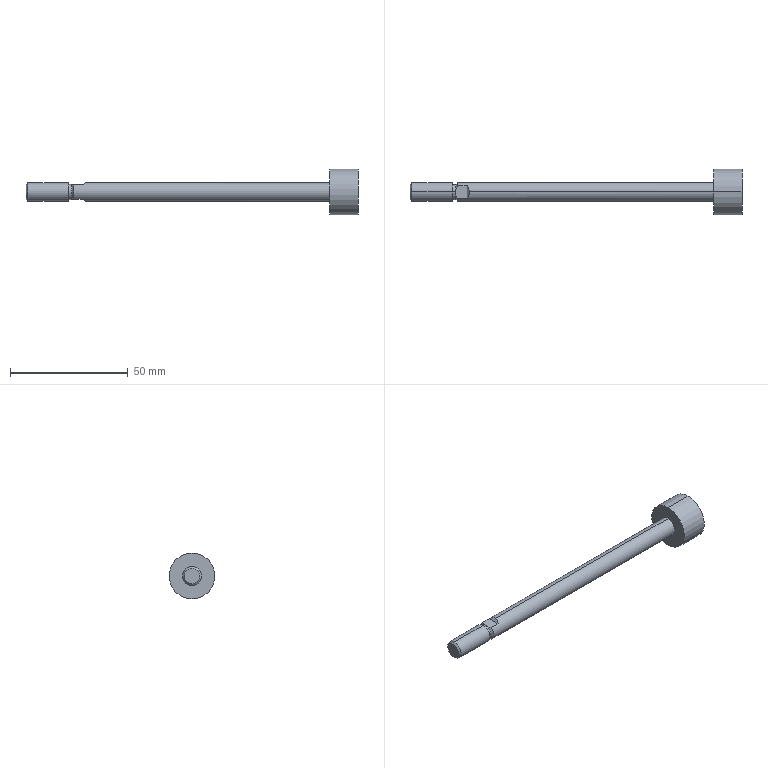Part | SolidWorks | features BaseBody 1 | 1 solid | 22 faces | box 141.2 x 19.5 x 19.5 mm | volume 10002 mm3 | plane 10 | cylinder 8 | cone 4 | commonest cylinder face diameters 8 x4 6.4 x2 19.5 x2
STEP:
#1=CARTESIAN_POINT('',(-24.5,-1.114,3.));
#2=VERTEX_POINT('',#1);
#3=CARTESIAN_POINT('',(-23.7,-2.646,3.));
#4=VERTEX_POINT('',#3);
#5=CARTESIAN_POINT('',(-24.5,-1.114,3.));
#6=CARTESIAN_POINT('',(-24.457,-1.239,3.));
#7=CARTESIAN_POINT('',(-24.38,-1.431,3.));
#8=CARTESIAN_POINT('',(-24.27,-1.665,3.));
#9=CARTESIAN_POINT('',(-24.21,-1.784,3.));
#10=CARTESIAN_POINT('',(-24.179,-1.844,3.));
#11=CARTESIAN_POINT('',(-24.165,-1.87,3.));
#12=CARTESIAN_POINT('',(-24.156,-1.887,3.));
#13=CARTESIAN_POINT('',(-24.151,-1.897,3.));
#14=CARTESIAN_POINT('',(-24.022,-2.137,3.));
#15=CARTESIAN_POINT('',(-23.873,-2.384,3.));
#16=CARTESIAN_POINT('',(-23.7,-2.646,3.));
#17=B_SPLINE_CURVE_WITH_KNOTS('',3,(#5,#6,#7,#8,#9,#10,#11,#12,#13,#14,#15,#16),.UNSPECIFIED.,.F.,.F.,(4,1,1,1,1,2,2,4),(0.,0.25,0.375,0.4375,0.4688,0.4844,0.5,1.),.UNSPECIFIED.);
#18=EDGE_CURVE('',#2,#4,#17,.T.);
#19=ORIENTED_EDGE('',*,*,#18,.T.);
#20=CARTESIAN_POINT('',(-19.7,-2.646,3.));
#21=VERTEX_POINT('',#20);
#22=CARTESIAN_POINT('',(-23.7,-2.646,3.));
#23=DIRECTION('',(1.,0.,0.));
#24=VECTOR('',#23,1000.);
#25=LINE('',#22,#24);
#26=EDGE_CURVE('',#4,#21,#25,.T.);
#27=ORIENTED_EDGE('',*,*,#26,.T.);
#28=CARTESIAN_POINT('',(-19.7,2.646,3.));
#29=VERTEX_POINT('',#28);
#30=CARTESIAN_POINT('',(-19.7,2.646,3.));
#31=DIRECTION('',(0.,-1.,0.));
#32=VECTOR('',#31,1000.);
#33=LINE('',#30,#32);
#34=EDGE_CURVE('',#29,#21,#33,.T.);
#35=ORIENTED_EDGE('',*,*,#34,.F.);
#36=CARTESIAN_POINT('',(-23.7,2.646,3.));
#37=VERTEX_POINT('',#36);
#38=CARTESIAN_POINT('',(-19.7,2.646,3.));
#39=DIRECTION('',(-1.,0.,0.));
#40=VECTOR('',#39,1000.);
#41=LINE('',#38,#40);
#42=EDGE_CURVE('',#29,#37,#41,.T.);
#43=ORIENTED_EDGE('',*,*,#42,.T.);
#44=CARTESIAN_POINT('',(-24.5,1.114,3.));
#45=VERTEX_POINT('',#44);
#46=CARTESIAN_POINT('',(-23.7,2.646,3.));
#47=CARTESIAN_POINT('',(-23.787,2.515,3.));
#48=CARTESIAN_POINT('',(-23.907,2.324,3.));
#49=CARTESIAN_POINT('',(-24.033,2.11,3.));
#50=CARTESIAN_POINT('',(-24.091,2.006,3.));
#51=CARTESIAN_POINT('',(-24.119,1.955,3.));
#52=CARTESIAN_POINT('',(-24.131,1.933,3.));
#53=CARTESIAN_POINT('',(-24.139,1.918,3.));
#54=CARTESIAN_POINT('',(-24.142,1.912,3.));
#55=CARTESIAN_POINT('',(-24.295,1.627,3.));
#56=CARTESIAN_POINT('',(-24.413,1.363,3.));
#57=CARTESIAN_POINT('',(-24.5,1.114,3.));
#58=B_SPLINE_CURVE_WITH_KNOTS('',3,(#46,#47,#48,#49,#50,#51,#52,#53,#54,#55,#56,#57),.UNSPECIFIED.,.F.,.F.,(4,1,1,1,1,2,2,4),(0.,0.25,0.375,0.4375,0.4688,0.4844,0.5,1.),.UNSPECIFIED.);
#59=EDGE_CURVE('',#37,#45,#58,.T.);
#60=ORIENTED_EDGE('',*,*,#59,.T.);
#61=CARTESIAN_POINT('',(-24.5,1.114,3.));
#62=DIRECTION('',(0.,-1.,0.));
#63=VECTOR('',#62,1000.);
#64=LINE('',#61,#63);
#65=EDGE_CURVE('',#45,#2,#64,.T.);
#66=ORIENTED_EDGE('',*,*,#65,.T.);
#67=EDGE_LOOP('',(#19,#27,#35,#43,#60,#66));
#68=FACE_OUTER_BOUND('',#67,.T.);
#69=CARTESIAN_POINT('',(-19.7,8.,3.));
#70=DIRECTION('',(0.,0.,1.));
#71=DIRECTION('',(1.,0.,0.));
#72=AXIS2_PLACEMENT_3D('',#69,#70,#71);
#73=PLANE('',#72);
#74=ADVANCED_FACE('',(#68),#73,.T.);
#75=CARTESIAN_POINT('',(-18.7,0.,4.));
#76=VERTEX_POINT('',#75);
#77=CARTESIAN_POINT('',(-19.7,-2.646,3.));
#78=CARTESIAN_POINT('',(-19.378,-2.281,3.322));
#79=CARTESIAN_POINT('',(-19.131,-1.87,3.569));
#80=CARTESIAN_POINT('',(-18.786,-0.9587,3.914));
#81=CARTESIAN_POINT('',(-18.7,-0.4873,4.));
#82=CARTESIAN_POINT('',(-18.7,0.,4.));
#83=B_SPLINE_CURVE_WITH_KNOTS('',3,(#77,#78,#79,#80,#81,#82),.UNSPECIFIED.,.F.,.F.,(4,2,4),(0.,0.5,1.),.UNSPECIFIED.);
#84=EDGE_CURVE('',#21,#76,#83,.T.);
#85=ORIENTED_EDGE('',*,*,#84,.T.);
#86=CARTESIAN_POINT('',(-18.7,0.,4.));
#87=CARTESIAN_POINT('',(-18.7,0.487,4.));
#88=CARTESIAN_POINT('',(-18.786,0.9587,3.914));
#89=CARTESIAN_POINT('',(-19.13,1.87,3.57));
#90=CARTESIAN_POINT('',(-19.378,2.28,3.322));
#91=CARTESIAN_POINT('',(-19.7,2.646,3.));
#92=B_SPLINE_CURVE_WITH_KNOTS('',3,(#86,#87,#88,#89,#90,#91),.UNSPECIFIED.,.F.,.F.,(4,2,4),(0.,0.5,1.),.UNSPECIFIED.);
#93=EDGE_CURVE('',#76,#29,#92,.T.);
#94=ORIENTED_EDGE('',*,*,#93,.T.);
#95=ORIENTED_EDGE('',*,*,#34,.T.);
#96=EDGE_LOOP('',(#85,#94,#95));
#97=FACE_OUTER_BOUND('',#96,.T.);
#98=CARTESIAN_POINT('',(-13.7,8.,9.));
#99=DIRECTION('',(-0.7071,0.,0.7071));
#100=DIRECTION('',(0.,1.,0.));
#101=AXIS2_PLACEMENT_3D('',#98,#99,#100);
#102=PLANE('',#101);
#103=ADVANCED_FACE('',(#97),#102,.T.);
#104=CARTESIAN_POINT('',(-24.5,0.,3.2));
#105=VERTEX_POINT('',#104);
#106=CARTESIAN_POINT('',(-24.5,0.,0.));
#107=DIRECTION('',(1.,0.,0.));
#108=DIRECTION('',(0.,0.348,0.9375));
#109=AXIS2_PLACEMENT_3D('',#106,#107,#108);
#110=CIRCLE('',#109,3.2);
#111=EDGE_CURVE('',#45,#105,#110,.T.);
#112=ORIENTED_EDGE('',*,*,#111,.T.);
#113=CARTESIAN_POINT('',(-24.5,0.,0.));
#114=DIRECTION('',(1.,0.,0.));
#115=DIRECTION('',(0.,0.348,0.9375));
#116=AXIS2_PLACEMENT_3D('',#113,#114,#115);
#117=CIRCLE('',#116,3.2);
#118=EDGE_CURVE('',#105,#2,#117,.T.);
#119=ORIENTED_EDGE('',*,*,#118,.T.);
#120=ORIENTED_EDGE('',*,*,#65,.F.);
#121=EDGE_LOOP('',(#112,#119,#120));
#122=FACE_OUTER_BOUND('',#121,.T.);
#123=CARTESIAN_POINT('',(-24.5,8.,3.));
#124=DIRECTION('',(1.,0.,0.));
#125=DIRECTION('',(0.,1.,0.));
#126=AXIS2_PLACEMENT_3D('',#123,#124,#125);
#127=PLANE('',#126);
#128=ADVANCED_FACE('',(#122),#127,.T.);
#129=CARTESIAN_POINT('',(-24.5,-1.114,-3.));
#130=VERTEX_POINT('',#129);
#131=CARTESIAN_POINT('',(-24.5,0.,-3.2));
#132=VERTEX_POINT('',#131);
#133=CARTESIAN_POINT('',(-24.5,0.,0.));
#134=DIRECTION('',(1.,0.,0.));
#135=DIRECTION('',(0.,-0.348,-0.9375));
#136=AXIS2_PLACEMENT_3D('',#133,#134,#135);
#137=CIRCLE('',#136,3.2);
#138=EDGE_CURVE('',#130,#132,#137,.T.);
#139=ORIENTED_EDGE('',*,*,#138,.T.);
#140=CARTESIAN_POINT('',(-24.5,1.114,-3.));
#141=VERTEX_POINT('',#140);
#142=CARTESIAN_POINT('',(-24.5,0.,0.));
#143=DIRECTION('',(1.,0.,0.));
#144=DIRECTION('',(0.,-0.348,-0.9375));
#145=AXIS2_PLACEMENT_3D('',#142,#143,#144);
#146=CIRCLE('',#145,3.2);
#147=EDGE_CURVE('',#132,#141,#146,.T.);
#148=ORIENTED_EDGE('',*,*,#147,.T.);
#149=CARTESIAN_POINT('',(-24.5,1.114,-3.));
#150=DIRECTION('',(0.,-1.,0.));
#151=VECTOR('',#150,1000.);
#152=LINE('',#149,#151);
#153=EDGE_CURVE('',#141,#130,#152,.T.);
#154=ORIENTED_EDGE('',*,*,#153,.T.);
#155=EDGE_LOOP('',(#139,#148,#154));
#156=FACE_OUTER_BOUND('',#155,.T.);
#157=CARTESIAN_POINT('',(-24.5,8.,-4.8));
#158=DIRECTION('',(1.,0.,0.));
#159=DIRECTION('',(0.,1.,0.));
#160=AXIS2_PLACEMENT_3D('',#157,#158,#159);
#161=PLANE('',#160);
#162=ADVANCED_FACE('',(#156),#161,.T.);
#163=CARTESIAN_POINT('',(-23.7,2.646,-3.));
#164=VERTEX_POINT('',#163);
#165=CARTESIAN_POINT('',(-24.5,1.114,-3.));
#166=CARTESIAN_POINT('',(-24.457,1.239,-3.));
#167=CARTESIAN_POINT('',(-24.38,1.431,-3.));
#168=CARTESIAN_POINT('',(-24.27,1.665,-3.));
#169=CARTESIAN_POINT('',(-24.21,1.784,-3.));
#170=CARTESIAN_POINT('',(-24.179,1.844,-3.));
#171=CARTESIAN_POINT('',(-24.165,1.87,-3.));
#172=CARTESIAN_POINT('',(-24.156,1.887,-3.));
#173=CARTESIAN_POINT('',(-24.151,1.897,-3.));
#174=CARTESIAN_POINT('',(-24.022,2.137,-3.));
#175=CARTESIAN_POINT('',(-23.873,2.384,-3.));
#176=CARTESIAN_POINT('',(-23.7,2.646,-3.));
#177=B_SPLINE_CURVE_WITH_KNOTS('',3,(#165,#166,#167,#168,#169,#170,#171,#172,#173,#174,#175,#176),.UNSPECIFIED.,.F.,.F.,(4,1,1,1,1,2,2,4),(0.,0.25,0.375,0.4375,0.4687,0.4844,0.5,1.),.UNSPECIFIED.);
#178=EDGE_CURVE('',#141,#164,#177,.T.);
#179=ORIENTED_EDGE('',*,*,#178,.T.);
#180=CARTESIAN_POINT('',(-19.7,2.646,-3.));
#181=VERTEX_POINT('',#180);
#182=CARTESIAN_POINT('',(-23.7,2.646,-3.));
#183=DIRECTION('',(1.,0.,0.));
#184=VECTOR('',#183,1000.);
#185=LINE('',#182,#184);
#186=EDGE_CURVE('',#164,#181,#185,.T.);
#187=ORIENTED_EDGE('',*,*,#186,.T.);
#188=CARTESIAN_POINT('',(-19.7,-2.646,-3.));
#189=VERTEX_POINT('',#188);
#190=CARTESIAN_POINT('',(-19.7,2.646,-3.));
#191=DIRECTION('',(0.,-1.,0.));
#192=VECTOR('',#191,1000.);
#193=LINE('',#190,#192);
#194=EDGE_CURVE('',#181,#189,#193,.T.);
#195=ORIENTED_EDGE('',*,*,#194,.T.);
#196=CARTESIAN_POINT('',(-23.7,-2.646,-3.));
#197=VERTEX_POINT('',#196);
#198=CARTESIAN_POINT('',(-19.7,-2.646,-3.));
#199=DIRECTION('',(-1.,0.,0.));
#200=VECTOR('',#199,1000.);
#201=LINE('',#198,#200);
#202=EDGE_CURVE('',#189,#197,#201,.T.);
#203=ORIENTED_EDGE('',*,*,#202,.T.);
#204=CARTESIAN_POINT('',(-23.7,-2.646,-3.));
#205=CARTESIAN_POINT('',(-23.787,-2.515,-3.));
#206=CARTESIAN_POINT('',(-23.907,-2.324,-3.));
#207=CARTESIAN_POINT('',(-24.033,-2.11,-3.));
#208=CARTESIAN_POINT('',(-24.091,-2.006,-3.));
#209=CARTESIAN_POINT('',(-24.119,-1.955,-3.));
#210=CARTESIAN_POINT('',(-24.131,-1.933,-3.));
#211=CARTESIAN_POINT('',(-24.139,-1.918,-3.));
#212=CARTESIAN_POINT('',(-24.142,-1.912,-3.));
#213=CARTESIAN_POINT('',(-24.295,-1.627,-3.));
#214=CARTESIAN_POINT('',(-24.413,-1.363,-3.));
#215=CARTESIAN_POINT('',(-24.5,-1.114,-3.));
#216=B_SPLINE_CURVE_WITH_KNOTS('',3,(#204,#205,#206,#207,#208,#209,#210,#211,#212,#213,#214,#215),.UNSPECIFIED.,.F.,.F.,(4,1,1,1,1,2,2,4),(0.,0.25,0.375,0.4375,0.4687,0.4844,0.5,1.),.UNSPECIFIED.);
#217=EDGE_CURVE('',#197,#130,#216,.T.);
#218=ORIENTED_EDGE('',*,*,#217,.T.);
#219=ORIENTED_EDGE('',*,*,#153,.F.);
#220=EDGE_LOOP('',(#179,#187,#195,#203,#218,#219));
#221=FACE_OUTER_BOUND('',#220,.T.);
#222=CARTESIAN_POINT('',(-24.5,8.,-3.));
#223=DIRECTION('',(0.,0.,-1.));
#224=DIRECTION('',(0.,-1.,0.));
#225=AXIS2_PLACEMENT_3D('',#222,#223,#224);
#226=PLANE('',#225);
#227=ADVANCED_FACE('',(#221),#226,.T.);
#228=CARTESIAN_POINT('',(-18.7,0.,-4.));
#229=VERTEX_POINT('',#228);
#230=CARTESIAN_POINT('',(-19.7,2.646,-3.));
#231=CARTESIAN_POINT('',(-19.378,2.281,-3.322));
#232=CARTESIAN_POINT('',(-19.131,1.87,-3.569));
#233=CARTESIAN_POINT('',(-18.786,0.9587,-3.914));
#234=CARTESIAN_POINT('',(-18.7,0.4873,-4.));
#235=CARTESIAN_POINT('',(-18.7,0.,-4.));
#236=B_SPLINE_CURVE_WITH_KNOTS('',3,(#230,#231,#232,#233,#234,#235),.UNSPECIFIED.,.F.,.F.,(4,2,4),(0.,0.5,1.),.UNSPECIFIED.);
#237=EDGE_CURVE('',#181,#229,#236,.T.);
#238=ORIENTED_EDGE('',*,*,#237,.T.);
#239=CARTESIAN_POINT('',(-18.7,0.,-4.));
#240=CARTESIAN_POINT('',(-18.7,-0.487,-4.));
#241=CARTESIAN_POINT('',(-18.786,-0.9587,-3.914));
#242=CARTESIAN_POINT('',(-19.13,-1.87,-3.57));
#243=CARTESIAN_POINT('',(-19.378,-2.28,-3.322));
#244=CARTESIAN_POINT('',(-19.7,-2.646,-3.));
#245=B_SPLINE_CURVE_WITH_KNOTS('',3,(#239,#240,#241,#242,#243,#244),.UNSPECIFIED.,.F.,.F.,(4,2,4),(0.,0.5,1.),.UNSPECIFIED.);
#246=EDGE_CURVE('',#229,#189,#245,.T.);
#247=ORIENTED_EDGE('',*,*,#246,.T.);
#248=ORIENTED_EDGE('',*,*,#194,.F.);
#249=EDGE_LOOP('',(#238,#247,#248));
#250=FACE_OUTER_BOUND('',#249,.T.);
#251=CARTESIAN_POINT('',(-19.7,8.,-3.));
#252=DIRECTION('',(-0.7071,0.,-0.7071));
#253=DIRECTION('',(-0.7071,0.,0.7071));
#254=AXIS2_PLACEMENT_3D('',#251,#252,#253);
#255=PLANE('',#254);
#256=ADVANCED_FACE('',(#250),#255,.T.);
#257=CARTESIAN_POINT('',(97.2,0.,-9.75));
#258=VERTEX_POINT('',#257);
#259=CARTESIAN_POINT('',(97.2,0.,9.75));
#260=VERTEX_POINT('',#259);
#261=CARTESIAN_POINT('',(97.2,0.,0.));
#262=DIRECTION('',(1.,0.,0.));
#263=DIRECTION('',(0.,0.,-1.));
#264=AXIS2_PLACEMENT_3D('',#261,#262,#263);
#265=CIRCLE('',#264,9.75);
#266=EDGE_CURVE('',#258,#260,#265,.T.);
#267=ORIENTED_EDGE('',*,*,#266,.T.);
#268=CARTESIAN_POINT('',(97.2,0.,0.));
#269=DIRECTION('',(1.,0.,0.));
#270=DIRECTION('',(0.,0.,-1.));
#271=AXIS2_PLACEMENT_3D('',#268,#269,#270);
#272=CIRCLE('',#271,9.75);
#273=EDGE_CURVE('',#260,#258,#272,.T.);
#274=ORIENTED_EDGE('',*,*,#273,.T.);
#275=EDGE_LOOP('',(#267,#274));
#276=FACE_OUTER_BOUND('',#275,.T.);
#277=CARTESIAN_POINT('',(97.2,9.75,0.));
#278=DIRECTION('',(-1.,0.,0.));
#279=DIRECTION('',(0.,0.,1.));
#280=AXIS2_PLACEMENT_3D('',#277,#278,#279);
#281=PLANE('',#280);
#282=ADVANCED_FACE('',(#276),#281,.F.);
#283=CARTESIAN_POINT('',(85.2,0.,9.75));
#284=VERTEX_POINT('',#283);
#285=CARTESIAN_POINT('',(97.2,0.,9.75));
#286=DIRECTION('',(1.,0.,0.));
#287=VECTOR('',#286,1000.);
#288=LINE('',#285,#287);
#289=EDGE_CURVE('',#284,#260,#288,.T.);
#290=ORIENTED_EDGE('',*,*,#289,.F.);
#291=CARTESIAN_POINT('',(85.2,0.,-9.75));
#292=VERTEX_POINT('',#291);
#293=CARTESIAN_POINT('',(85.2,0.,0.));
#294=DIRECTION('',(1.,0.,0.));
#295=DIRECTION('',(0.,0.,-1.));
#296=AXIS2_PLACEMENT_3D('',#293,#294,#295);
#297=CIRCLE('',#296,9.75);
#298=EDGE_CURVE('',#284,#292,#297,.T.);
#299=ORIENTED_EDGE('',*,*,#298,.T.);
#300=CARTESIAN_POINT('',(97.2,0.,-9.75));
#301=DIRECTION('',(1.,0.,0.));
#302=VECTOR('',#301,1000.);
#303=LINE('',#300,#302);
#304=EDGE_CURVE('',#292,#258,#303,.T.);
#305=ORIENTED_EDGE('',*,*,#304,.T.);
#306=ORIENTED_EDGE('',*,*,#273,.F.);
#307=EDGE_LOOP('',(#290,#299,#305,#306));
#308=FACE_OUTER_BOUND('',#307,.T.);
#309=CARTESIAN_POINT('',(97.2,0.,0.));
#310=DIRECTION('',(1.,0.,0.));
#311=DIRECTION('',(0.,0.,-1.));
#312=AXIS2_PLACEMENT_3D('',#309,#310,#311);
#313=CYLINDRICAL_SURFACE('',#312,9.75);
#314=ADVANCED_FACE('',(#308),#313,.T.);
#315=CARTESIAN_POINT('',(85.2,0.,-4.));
#316=VERTEX_POINT('',#315);
#317=CARTESIAN_POINT('',(85.2,0.,4.));
#318=VERTEX_POINT('',#317);
#319=CARTESIAN_POINT('',(85.2,0.,0.));
#320=DIRECTION('',(1.,0.,0.));
#321=DIRECTION('',(0.,0.,-1.));
#322=AXIS2_PLACEMENT_3D('',#319,#320,#321);
#323=CIRCLE('',#322,4.);
#324=EDGE_CURVE('',#316,#318,#323,.T.);
#325=ORIENTED_EDGE('',*,*,#324,.T.);
#326=CARTESIAN_POINT('',(85.2,0.,0.));
#327=DIRECTION('',(1.,0.,0.));
#328=DIRECTION('',(0.,0.,-1.));
#329=AXIS2_PLACEMENT_3D('',#326,#327,#328);
#330=CIRCLE('',#329,4.);
#331=EDGE_CURVE('',#318,#316,#330,.T.);
#332=ORIENTED_EDGE('',*,*,#331,.T.);
#333=EDGE_LOOP('',(#325,#332));
#334=FACE_BOUND('',#333,.T.);
#335=CARTESIAN_POINT('',(85.2,0.,0.));
#336=DIRECTION('',(1.,0.,0.));
#337=DIRECTION('',(0.,0.,-1.));
#338=AXIS2_PLACEMENT_3D('',#335,#336,#337);
#339=CIRCLE('',#338,9.75);
#340=EDGE_CURVE('',#292,#284,#339,.T.);
#341=ORIENTED_EDGE('',*,*,#340,.F.);
#342=ORIENTED_EDGE('',*,*,#298,.F.);
#343=EDGE_LOOP('',(#341,#342));
#344=FACE_OUTER_BOUND('',#343,.T.);
#345=CARTESIAN_POINT('',(85.2,4.,0.));
#346=DIRECTION('',(1.,0.,0.));
#347=DIRECTION('',(0.,1.,0.));
#348=AXIS2_PLACEMENT_3D('',#345,#346,#347);
#349=PLANE('',#348);
#350=ADVANCED_FACE('',(#334,#344),#349,.F.);
#351=CARTESIAN_POINT('',(-26.,0.,3.2));
#352=VERTEX_POINT('',#351);
#353=CARTESIAN_POINT('',(97.2,0.,3.2));
#354=DIRECTION('',(1.,0.,0.));
#355=VECTOR('',#354,1000.);
#356=LINE('',#353,#355);
#357=EDGE_CURVE('',#352,#105,#356,.T.);
#358=ORIENTED_EDGE('',*,*,#357,.F.);
#359=CARTESIAN_POINT('',(-26.,0.,-3.2));
#360=VERTEX_POINT('',#359);
#361=CARTESIAN_POINT('',(-26.,0.,0.));
#362=DIRECTION('',(1.,0.,0.));
#363=DIRECTION('',(0.,0.,-1.));
#364=AXIS2_PLACEMENT_3D('',#361,#362,#363);
#365=CIRCLE('',#364,3.2);
#366=EDGE_CURVE('',#352,#360,#365,.T.);
#367=ORIENTED_EDGE('',*,*,#366,.T.);
#368=CARTESIAN_POINT('',(97.2,0.,-3.2));
#369=DIRECTION('',(1.,0.,0.));
#370=VECTOR('',#369,1000.);
#371=LINE('',#368,#370);
#372=EDGE_CURVE('',#360,#132,#371,.T.);
#373=ORIENTED_EDGE('',*,*,#372,.T.);
#374=ORIENTED_EDGE('',*,*,#138,.F.);
#375=CARTESIAN_POINT('',(-24.5,0.,0.));
#376=DIRECTION('',(1.,0.,0.));
#377=DIRECTION('',(0.,-0.348,0.9375));
#378=AXIS2_PLACEMENT_3D('',#375,#376,#377);
#379=CIRCLE('',#378,3.2);
#380=EDGE_CURVE('',#2,#130,#379,.T.);
#381=ORIENTED_EDGE('',*,*,#380,.F.);
#382=ORIENTED_EDGE('',*,*,#118,.F.);
#383=EDGE_LOOP('',(#358,#367,#373,#374,#381,#382));
#384=FACE_OUTER_BOUND('',#383,.T.);
#385=CARTESIAN_POINT('',(97.2,0.,0.));
#386=DIRECTION('',(1.,0.,0.));
#387=DIRECTION('',(0.,0.,-1.));
#388=AXIS2_PLACEMENT_3D('',#385,#386,#387);
#389=CYLINDRICAL_SURFACE('',#388,3.2);
#390=ADVANCED_FACE('',(#384),#389,.T.);
#391=CARTESIAN_POINT('',(-26.,0.,0.));
#392=DIRECTION('',(1.,0.,0.));
#393=DIRECTION('',(0.,0.,-1.));
#394=AXIS2_PLACEMENT_3D('',#391,#392,#393);
#395=CIRCLE('',#394,3.2);
#396=EDGE_CURVE('',#360,#352,#395,.T.);
#397=ORIENTED_EDGE('',*,*,#396,.F.);
#398=ORIENTED_EDGE('',*,*,#366,.F.);
#399=EDGE_LOOP('',(#397,#398));
#400=FACE_BOUND('',#399,.T.);
#401=CARTESIAN_POINT('',(-26.,0.,-4.));
#402=VERTEX_POINT('',#401);
#403=CARTESIAN_POINT('',(-26.,0.,4.));
#404=VERTEX_POINT('',#403);
#405=CARTESIAN_POINT('',(-26.,0.,0.));
#406=DIRECTION('',(1.,0.,0.));
#407=DIRECTION('',(0.,0.,-1.));
#408=AXIS2_PLACEMENT_3D('',#405,#406,#407);
#409=CIRCLE('',#408,4.);
#410=EDGE_CURVE('',#402,#404,#409,.T.);
#411=ORIENTED_EDGE('',*,*,#410,.T.);
#412=CARTESIAN_POINT('',(-26.,0.,0.));
#413=DIRECTION('',(1.,0.,0.));
#414=DIRECTION('',(0.,0.,-1.));
#415=AXIS2_PLACEMENT_3D('',#412,#413,#414);
#416=CIRCLE('',#415,4.);
#417=EDGE_CURVE('',#404,#402,#416,.T.);
#418=ORIENTED_EDGE('',*,*,#417,.T.);
#419=EDGE_LOOP('',(#411,#418));
#420=FACE_OUTER_BOUND('',#419,.T.);
#421=CARTESIAN_POINT('',(-26.,4.,0.));
#422=DIRECTION('',(-1.,0.,0.));
#423=DIRECTION('',(0.,0.,1.));
#424=AXIS2_PLACEMENT_3D('',#421,#422,#423);
#425=PLANE('',#424);
#426=ADVANCED_FACE('',(#400,#420),#425,.F.);
#427=CARTESIAN_POINT('',(-43.233,0.,4.));
#428=VERTEX_POINT('',#427);
#429=CARTESIAN_POINT('',(97.2,0.,4.));
#430=DIRECTION('',(1.,0.,0.));
#431=VECTOR('',#430,1000.);
#432=LINE('',#429,#431);
#433=EDGE_CURVE('',#428,#404,#432,.T.);
#434=ORIENTED_EDGE('',*,*,#433,.F.);
#435=CARTESIAN_POINT('',(-43.233,0.,-4.));
#436=VERTEX_POINT('',#435);
#437=CARTESIAN_POINT('',(-43.233,0.,0.));
#438=DIRECTION('',(1.,0.,0.));
#439=DIRECTION('',(0.,0.,-1.));
#440=AXIS2_PLACEMENT_3D('',#437,#438,#439);
#441=CIRCLE('',#440,4.);
#442=EDGE_CURVE('',#428,#436,#441,.T.);
#443=ORIENTED_EDGE('',*,*,#442,.T.);
#444=CARTESIAN_POINT('',(97.2,0.,-4.));
#445=DIRECTION('',(1.,0.,0.));
#446=VECTOR('',#445,1000.);
#447=LINE('',#444,#446);
#448=EDGE_CURVE('',#436,#402,#447,.T.);
#449=ORIENTED_EDGE('',*,*,#448,.T.);
#450=ORIENTED_EDGE('',*,*,#417,.F.);
#451=EDGE_LOOP('',(#434,#443,#449,#450));
#452=FACE_OUTER_BOUND('',#451,.T.);
#453=CARTESIAN_POINT('',(97.2,0.,0.));
#454=DIRECTION('',(1.,0.,0.));
#455=DIRECTION('',(0.,0.,-1.));
#456=AXIS2_PLACEMENT_3D('',#453,#454,#455);
#457=CYLINDRICAL_SURFACE('',#456,4.);
#458=ADVANCED_FACE('',(#452),#457,.T.);
#459=CARTESIAN_POINT('',(-44.,0.,3.233));
#460=VERTEX_POINT('',#459);
#461=CARTESIAN_POINT('',(-44.,0.,3.233));
#462=DIRECTION('',(0.7071,0.,0.7071));
#463=VECTOR('',#462,1000.);
#464=LINE('',#461,#463);
#465=EDGE_CURVE('',#460,#428,#464,.T.);
#466=ORIENTED_EDGE('',*,*,#465,.F.);
#467=CARTESIAN_POINT('',(-44.,0.,-3.233));
#468=VERTEX_POINT('',#467);
#469=CARTESIAN_POINT('',(-44.,0.,0.));
#470=DIRECTION('',(1.,0.,0.));
#471=DIRECTION('',(0.,0.,-1.));
#472=AXIS2_PLACEMENT_3D('',#469,#470,#471);
#473=CIRCLE('',#472,3.233);
#474=EDGE_CURVE('',#460,#468,#473,.T.);
#475=ORIENTED_EDGE('',*,*,#474,.T.);
#476=CARTESIAN_POINT('',(-44.,0.,-3.233));
#477=DIRECTION('',(0.7071,0.,-0.7071));
#478=VECTOR('',#477,1000.);
#479=LINE('',#476,#478);
#480=EDGE_CURVE('',#468,#436,#479,.T.);
#481=ORIENTED_EDGE('',*,*,#480,.T.);
#482=ORIENTED_EDGE('',*,*,#442,.F.);
#483=EDGE_LOOP('',(#466,#475,#481,#482));
#484=FACE_OUTER_BOUND('',#483,.T.);
#485=CARTESIAN_POINT('',(-44.,0.,0.));
#486=DIRECTION('',(1.,0.,0.));
#487=DIRECTION('',(0.,0.,-1.));
#488=AXIS2_PLACEMENT_3D('',#485,#486,#487);
#489=CONICAL_SURFACE('',#488,3.233,0.7854);
#490=ADVANCED_FACE('',(#484),#489,.T.);
#491=CARTESIAN_POINT('',(-44.,0.,0.));
#492=DIRECTION('',(1.,0.,0.));
#493=DIRECTION('',(0.,0.,-1.));
#494=AXIS2_PLACEMENT_3D('',#491,#492,#493);
#495=CIRCLE('',#494,3.233);
#496=EDGE_CURVE('',#468,#460,#495,.T.);
#497=ORIENTED_EDGE('',*,*,#496,.F.);
#498=ORIENTED_EDGE('',*,*,#474,.F.);
#499=EDGE_LOOP('',(#497,#498));
#500=FACE_OUTER_BOUND('',#499,.T.);
#501=CARTESIAN_POINT('',(-44.,0.,0.));
#502=DIRECTION('',(1.,0.,0.));
#503=DIRECTION('',(0.,1.,0.));
#504=AXIS2_PLACEMENT_3D('',#501,#502,#503);
#505=PLANE('',#504);
#506=ADVANCED_FACE('',(#500),#505,.F.);
#507=CARTESIAN_POINT('',(97.2,0.,4.));
#508=DIRECTION('',(1.,0.,0.));
#509=VECTOR('',#508,1000.);
#510=LINE('',#507,#509);
#511=EDGE_CURVE('',#76,#318,#510,.T.);
#512=ORIENTED_EDGE('',*,*,#511,.F.);
#513=ORIENTED_EDGE('',*,*,#84,.F.);
#514=ORIENTED_EDGE('',*,*,#26,.F.);
#515=CARTESIAN_POINT('',(-23.7,0.,0.));
#516=DIRECTION('',(1.,0.,0.));
#517=DIRECTION('',(0.,-0.6614,0.75));
#518=AXIS2_PLACEMENT_3D('',#515,#516,#517);
#519=CIRCLE('',#518,4.);
#520=EDGE_CURVE('',#4,#197,#519,.T.);
#521=ORIENTED_EDGE('',*,*,#520,.T.);
#522=ORIENTED_EDGE('',*,*,#202,.F.);
#523=ORIENTED_EDGE('',*,*,#246,.F.);
#524=CARTESIAN_POINT('',(97.2,0.,-4.));
#525=DIRECTION('',(1.,0.,0.));
#526=VECTOR('',#525,1000.);
#527=LINE('',#524,#526);
#528=EDGE_CURVE('',#229,#316,#527,.T.);
#529=ORIENTED_EDGE('',*,*,#528,.T.);
#530=ORIENTED_EDGE('',*,*,#331,.F.);
#531=EDGE_LOOP('',(#512,#513,#514,#521,#522,#523,#529,#530));
#532=FACE_OUTER_BOUND('',#531,.T.);
#533=CARTESIAN_POINT('',(97.2,0.,0.));
#534=DIRECTION('',(1.,0.,0.));
#535=DIRECTION('',(0.,0.,-1.));
#536=AXIS2_PLACEMENT_3D('',#533,#534,#535);
#537=CYLINDRICAL_SURFACE('',#536,4.);
#538=ADVANCED_FACE('',(#532),#537,.T.);
#539=ORIENTED_EDGE('',*,*,#18,.F.);
#540=ORIENTED_EDGE('',*,*,#380,.T.);
#541=ORIENTED_EDGE('',*,*,#217,.F.);
#542=ORIENTED_EDGE('',*,*,#520,.F.);
#543=EDGE_LOOP('',(#539,#540,#541,#542));
#544=FACE_OUTER_BOUND('',#543,.T.);
#545=CARTESIAN_POINT('',(-24.5,0.,0.));
#546=DIRECTION('',(1.,0.,0.));
#547=DIRECTION('',(0.,0.,-1.));
#548=AXIS2_PLACEMENT_3D('',#545,#546,#547);
#549=CONICAL_SURFACE('',#548,3.2,0.7854);
#550=ADVANCED_FACE('',(#544),#549,.T.);
#551=ORIENTED_EDGE('',*,*,#59,.F.);
#552=CARTESIAN_POINT('',(-23.7,0.,0.));
#553=DIRECTION('',(1.,0.,0.));
#554=DIRECTION('',(0.,0.6614,-0.75));
#555=AXIS2_PLACEMENT_3D('',#552,#553,#554);
#556=CIRCLE('',#555,4.);
#557=EDGE_CURVE('',#164,#37,#556,.T.);
#558=ORIENTED_EDGE('',*,*,#557,.F.);
#559=ORIENTED_EDGE('',*,*,#178,.F.);
#560=CARTESIAN_POINT('',(-24.5,0.,0.));
#561=DIRECTION('',(1.,0.,0.));
#562=DIRECTION('',(0.,0.348,-0.9375));
#563=AXIS2_PLACEMENT_3D('',#560,#561,#562);
#564=CIRCLE('',#563,3.2);
#565=EDGE_CURVE('',#141,#45,#564,.T.);
#566=ORIENTED_EDGE('',*,*,#565,.T.);
#567=EDGE_LOOP('',(#551,#558,#559,#566));
#568=FACE_OUTER_BOUND('',#567,.T.);
#569=CARTESIAN_POINT('',(-24.5,0.,0.));
#570=DIRECTION('',(1.,0.,0.));
#571=DIRECTION('',(0.,0.,-1.));
#572=AXIS2_PLACEMENT_3D('',#569,#570,#571);
#573=CONICAL_SURFACE('',#572,3.2,0.7854);
#574=ADVANCED_FACE('',(#568),#573,.T.);
#575=ORIENTED_EDGE('',*,*,#93,.F.);
#576=ORIENTED_EDGE('',*,*,#511,.T.);
#577=ORIENTED_EDGE('',*,*,#324,.F.);
#578=ORIENTED_EDGE('',*,*,#528,.F.);
#579=ORIENTED_EDGE('',*,*,#237,.F.);
#580=ORIENTED_EDGE('',*,*,#186,.F.);
#581=ORIENTED_EDGE('',*,*,#557,.T.);
#582=ORIENTED_EDGE('',*,*,#42,.F.);
#583=EDGE_LOOP('',(#575,#576,#577,#578,#579,#580,#581,#582));
#584=FACE_OUTER_BOUND('',#583,.T.);
#585=CARTESIAN_POINT('',(97.2,0.,0.));
#586=DIRECTION('',(1.,0.,0.));
#587=DIRECTION('',(0.,0.,-1.));
#588=AXIS2_PLACEMENT_3D('',#585,#586,#587);
#589=CYLINDRICAL_SURFACE('',#588,4.);
#590=ADVANCED_FACE('',(#584),#589,.T.);
#591=ORIENTED_EDGE('',*,*,#496,.T.);
#592=ORIENTED_EDGE('',*,*,#465,.T.);
#593=CARTESIAN_POINT('',(-43.233,0.,0.));
#594=DIRECTION('',(1.,0.,0.));
#595=DIRECTION('',(0.,0.,-1.));
#596=AXIS2_PLACEMENT_3D('',#593,#594,#595);
#597=CIRCLE('',#596,4.);
#598=EDGE_CURVE('',#436,#428,#597,.T.);
#599=ORIENTED_EDGE('',*,*,#598,.F.);
#600=ORIENTED_EDGE('',*,*,#480,.F.);
#601=EDGE_LOOP('',(#591,#592,#599,#600));
#602=FACE_OUTER_BOUND('',#601,.T.);
#603=CARTESIAN_POINT('',(-44.,0.,0.));
#604=DIRECTION('',(1.,0.,0.));
#605=DIRECTION('',(0.,0.,-1.));
#606=AXIS2_PLACEMENT_3D('',#603,#604,#605);
#607=CONICAL_SURFACE('',#606,3.233,0.7854);
#608=ADVANCED_FACE('',(#602),#607,.T.);
#609=ORIENTED_EDGE('',*,*,#598,.T.);
#610=ORIENTED_EDGE('',*,*,#433,.T.);
#611=ORIENTED_EDGE('',*,*,#410,.F.);
#612=ORIENTED_EDGE('',*,*,#448,.F.);
#613=EDGE_LOOP('',(#609,#610,#611,#612));
#614=FACE_OUTER_BOUND('',#613,.T.);
#615=CARTESIAN_POINT('',(97.2,0.,0.));
#616=DIRECTION('',(1.,0.,0.));
#617=DIRECTION('',(0.,0.,-1.));
#618=AXIS2_PLACEMENT_3D('',#615,#616,#617);
#619=CYLINDRICAL_SURFACE('',#618,4.);
#620=ADVANCED_FACE('',(#614),#619,.T.);
#621=ORIENTED_EDGE('',*,*,#396,.T.);
#622=ORIENTED_EDGE('',*,*,#357,.T.);
#623=ORIENTED_EDGE('',*,*,#111,.F.);
#624=ORIENTED_EDGE('',*,*,#565,.F.);
#625=ORIENTED_EDGE('',*,*,#147,.F.);
#626=ORIENTED_EDGE('',*,*,#372,.F.);
#627=EDGE_LOOP('',(#621,#622,#623,#624,#625,#626));
#628=FACE_OUTER_BOUND('',#627,.T.);
#629=CARTESIAN_POINT('',(97.2,0.,0.));
#630=DIRECTION('',(1.,0.,0.));
#631=DIRECTION('',(0.,0.,-1.));
#632=AXIS2_PLACEMENT_3D('',#629,#630,#631);
#633=CYLINDRICAL_SURFACE('',#632,3.2);
#634=ADVANCED_FACE('',(#628),#633,.T.);
#635=ORIENTED_EDGE('',*,*,#340,.T.);
#636=ORIENTED_EDGE('',*,*,#289,.T.);
#637=ORIENTED_EDGE('',*,*,#266,.F.);
#638=ORIENTED_EDGE('',*,*,#304,.F.);
#639=EDGE_LOOP('',(#635,#636,#637,#638));
#640=FACE_OUTER_BOUND('',#639,.T.);
#641=CARTESIAN_POINT('',(97.2,0.,0.));
#642=DIRECTION('',(1.,0.,0.));
#643=DIRECTION('',(0.,0.,-1.));
#644=AXIS2_PLACEMENT_3D('',#641,#642,#643);
#645=CYLINDRICAL_SURFACE('',#644,9.75);
#646=ADVANCED_FACE('',(#640),#645,.T.);
#647=CLOSED_SHELL('',(#74,#103,#128,#162,#227,#256,#282,#314,#350,#390,#426,#458,#490,#506,#538,#550,#574,#590,#608,#620,#634,#646));
#648=MANIFOLD_SOLID_BREP('',#647);
#649=CARTESIAN_POINT('',(0.,0.,0.));
#650=DIRECTION('',(0.,0.,1.));
#651=DIRECTION('',(1.,0.,0.));
#652=AXIS2_PLACEMENT_3D('',#649,#650,#651);
#653=(LENGTH_UNIT()NAMED_UNIT(*)SI_UNIT(.MILLI.,.METRE.));
#654=UNCERTAINTY_MEASURE_WITH_UNIT(LENGTH_MEASURE(0.00001),#653,'','');
#655=(NAMED_UNIT(*)PLANE_ANGLE_UNIT()SI_UNIT($,.RADIAN.));
#656=(NAMED_UNIT(*)SI_UNIT($,.STERADIAN.)SOLID_ANGLE_UNIT());
#657=(GEOMETRIC_REPRESENTATION_CONTEXT(3)GLOBAL_UNCERTAINTY_ASSIGNED_CONTEXT((#654))GLOBAL_UNIT_ASSIGNED_CONTEXT((#653,#655,#656))REPRESENTATION_CONTEXT('',''));
#658=ADVANCED_BREP_SHAPE_REPRESENTATION('',(#648,#652),#657);